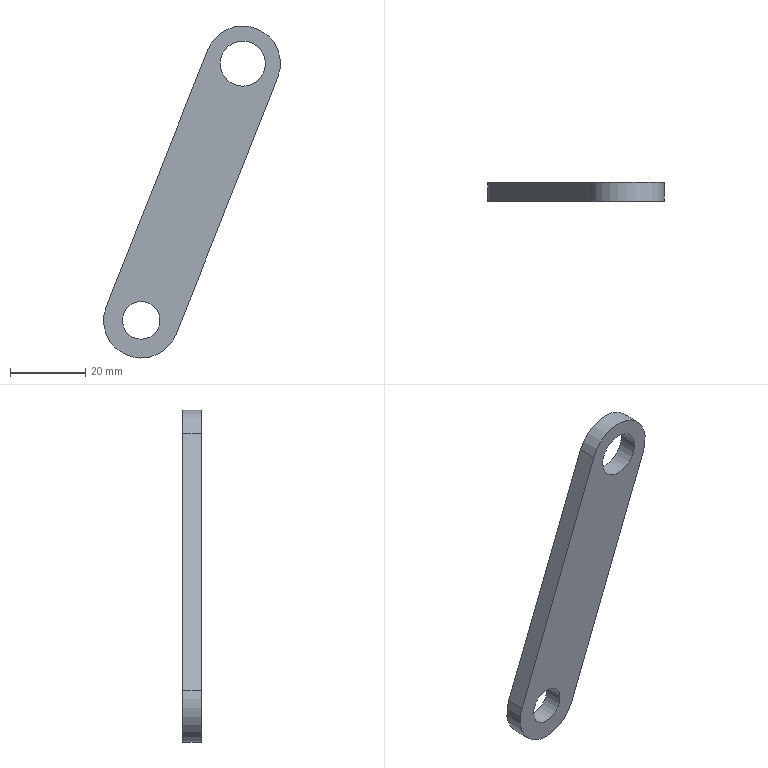Part | STEP file | 冲床-300配套压波_id290_x_t | 1 solid | 8 faces | box 47 x 5 x 88.25 mm | volume 7952 mm3 | cylinder 4 | plane 4 | commonest cylinder face diameters 20 x2 10 x1 12 x1
STEP:
#1=CARTESIAN_POINT('',(1139.299,-32.,157.071));
#2=VERTEX_POINT('',#1);
#3=CARTESIAN_POINT('',(1120.701,-32.,164.429));
#4=VERTEX_POINT('',#3);
#5=CARTESIAN_POINT('',(1130.,-32.,160.75));
#6=DIRECTION('',(0.,1.,0.));
#7=DIRECTION('',(1.,0.,0.));
#8=AXIS2_PLACEMENT_3D('',#5,#6,#7);
#9=CIRCLE('',#8,10.);
#10=EDGE_CURVE('',#2,#4,#9,.T.);
#11=ORIENTED_EDGE('',*,*,#10,.F.);
#12=CARTESIAN_POINT('',(1139.299,-37.,157.071));
#13=VERTEX_POINT('',#12);
#14=CARTESIAN_POINT('',(1139.299,-37.,157.071));
#15=DIRECTION('',(0.,1.,0.));
#16=VECTOR('',#15,1.);
#17=LINE('',#14,#16);
#18=EDGE_CURVE('',#13,#2,#17,.T.);
#19=ORIENTED_EDGE('',*,*,#18,.F.);
#20=CARTESIAN_POINT('',(1120.701,-37.,164.429));
#21=VERTEX_POINT('',#20);
#22=CARTESIAN_POINT('',(1130.,-37.,160.75));
#23=DIRECTION('',(0.,1.,0.));
#24=DIRECTION('',(1.,0.,0.));
#25=AXIS2_PLACEMENT_3D('',#22,#23,#24);
#26=CIRCLE('',#25,10.);
#27=EDGE_CURVE('',#13,#21,#26,.T.);
#28=ORIENTED_EDGE('',*,*,#27,.T.);
#29=CARTESIAN_POINT('',(1120.701,-37.,164.429));
#30=DIRECTION('',(0.,1.,0.));
#31=VECTOR('',#30,1.);
#32=LINE('',#29,#31);
#33=EDGE_CURVE('',#21,#4,#32,.T.);
#34=ORIENTED_EDGE('',*,*,#33,.T.);
#35=EDGE_LOOP('',(#11,#19,#28,#34));
#36=FACE_OUTER_BOUND('',#35,.T.);
#37=CARTESIAN_POINT('',(1130.,-37.,160.75));
#38=DIRECTION('',(0.,1.,0.));
#39=DIRECTION('',(0.,0.,1.));
#40=AXIS2_PLACEMENT_3D('',#37,#38,#39);
#41=CYLINDRICAL_SURFACE('',#40,10.);
#42=ADVANCED_FACE('',(#36),#41,.T.);
#43=CARTESIAN_POINT('',(1147.701,-32.,232.679));
#44=VERTEX_POINT('',#43);
#45=CARTESIAN_POINT('',(1120.701,-32.,164.429));
#46=DIRECTION('',(0.3679,0.,0.9299));
#47=VECTOR('',#46,1.);
#48=LINE('',#45,#47);
#49=EDGE_CURVE('',#4,#44,#48,.T.);
#50=ORIENTED_EDGE('',*,*,#49,.F.);
#51=ORIENTED_EDGE('',*,*,#33,.F.);
#52=CARTESIAN_POINT('',(1147.701,-37.,232.679));
#53=VERTEX_POINT('',#52);
#54=CARTESIAN_POINT('',(1120.701,-37.,164.429));
#55=DIRECTION('',(0.3679,0.,0.9299));
#56=VECTOR('',#55,1.);
#57=LINE('',#54,#56);
#58=EDGE_CURVE('',#21,#53,#57,.T.);
#59=ORIENTED_EDGE('',*,*,#58,.T.);
#60=CARTESIAN_POINT('',(1147.701,-37.,232.679));
#61=DIRECTION('',(0.,1.,0.));
#62=VECTOR('',#61,1.);
#63=LINE('',#60,#62);
#64=EDGE_CURVE('',#53,#44,#63,.T.);
#65=ORIENTED_EDGE('',*,*,#64,.T.);
#66=EDGE_LOOP('',(#50,#51,#59,#65));
#67=FACE_OUTER_BOUND('',#66,.T.);
#68=CARTESIAN_POINT('',(1120.701,-37.,164.429));
#69=DIRECTION('',(-0.9299,0.,0.3679));
#70=DIRECTION('',(0.3679,0.,0.9299));
#71=AXIS2_PLACEMENT_3D('',#68,#69,#70);
#72=PLANE('',#71);
#73=ADVANCED_FACE('',(#67),#72,.T.);
#74=CARTESIAN_POINT('',(1166.299,-32.,225.321));
#75=VERTEX_POINT('',#74);
#76=CARTESIAN_POINT('',(1157.,-32.,229.));
#77=DIRECTION('',(0.,1.,0.));
#78=DIRECTION('',(1.,0.,0.));
#79=AXIS2_PLACEMENT_3D('',#76,#77,#78);
#80=CIRCLE('',#79,10.);
#81=EDGE_CURVE('',#44,#75,#80,.T.);
#82=ORIENTED_EDGE('',*,*,#81,.F.);
#83=ORIENTED_EDGE('',*,*,#64,.F.);
#84=CARTESIAN_POINT('',(1166.299,-37.,225.321));
#85=VERTEX_POINT('',#84);
#86=CARTESIAN_POINT('',(1157.,-37.,229.));
#87=DIRECTION('',(0.,1.,0.));
#88=DIRECTION('',(1.,0.,0.));
#89=AXIS2_PLACEMENT_3D('',#86,#87,#88);
#90=CIRCLE('',#89,10.);
#91=EDGE_CURVE('',#53,#85,#90,.T.);
#92=ORIENTED_EDGE('',*,*,#91,.T.);
#93=CARTESIAN_POINT('',(1166.299,-37.,225.321));
#94=DIRECTION('',(0.,1.,0.));
#95=VECTOR('',#94,1.);
#96=LINE('',#93,#95);
#97=EDGE_CURVE('',#85,#75,#96,.T.);
#98=ORIENTED_EDGE('',*,*,#97,.T.);
#99=EDGE_LOOP('',(#82,#83,#92,#98));
#100=FACE_OUTER_BOUND('',#99,.T.);
#101=CARTESIAN_POINT('',(1157.,-37.,229.));
#102=DIRECTION('',(0.,1.,0.));
#103=DIRECTION('',(0.,0.,1.));
#104=AXIS2_PLACEMENT_3D('',#101,#102,#103);
#105=CYLINDRICAL_SURFACE('',#104,10.);
#106=ADVANCED_FACE('',(#100),#105,.T.);
#107=CARTESIAN_POINT('',(1166.299,-32.,225.321));
#108=DIRECTION('',(-0.3679,0.,-0.9299));
#109=VECTOR('',#108,1.);
#110=LINE('',#107,#109);
#111=EDGE_CURVE('',#75,#2,#110,.T.);
#112=ORIENTED_EDGE('',*,*,#111,.F.);
#113=ORIENTED_EDGE('',*,*,#97,.F.);
#114=CARTESIAN_POINT('',(1166.299,-37.,225.321));
#115=DIRECTION('',(-0.3679,0.,-0.9299));
#116=VECTOR('',#115,1.);
#117=LINE('',#114,#116);
#118=EDGE_CURVE('',#85,#13,#117,.T.);
#119=ORIENTED_EDGE('',*,*,#118,.T.);
#120=ORIENTED_EDGE('',*,*,#18,.T.);
#121=EDGE_LOOP('',(#112,#113,#119,#120));
#122=FACE_OUTER_BOUND('',#121,.T.);
#123=CARTESIAN_POINT('',(1166.299,-37.,225.321));
#124=DIRECTION('',(0.9299,0.,-0.3679));
#125=DIRECTION('',(-0.3679,0.,-0.9299));
#126=AXIS2_PLACEMENT_3D('',#123,#124,#125);
#127=PLANE('',#126);
#128=ADVANCED_FACE('',(#122),#127,.T.);
#129=CARTESIAN_POINT('',(1130.,-37.,165.75));
#130=VERTEX_POINT('',#129);
#131=CARTESIAN_POINT('',(1130.,-37.,160.75));
#132=DIRECTION('',(0.,-1.,0.));
#133=DIRECTION('',(0.,0.,1.));
#134=AXIS2_PLACEMENT_3D('',#131,#132,#133);
#135=CIRCLE('',#134,5.);
#136=EDGE_CURVE('',#130,#130,#135,.T.);
#137=ORIENTED_EDGE('',*,*,#136,.F.);
#138=EDGE_LOOP('',(#137));
#139=FACE_BOUND('',#138,.T.);
#140=CARTESIAN_POINT('',(1157.,-37.,235.));
#141=VERTEX_POINT('',#140);
#142=CARTESIAN_POINT('',(1157.,-37.,229.));
#143=DIRECTION('',(0.,-1.,0.));
#144=DIRECTION('',(0.,0.,1.));
#145=AXIS2_PLACEMENT_3D('',#142,#143,#144);
#146=CIRCLE('',#145,6.);
#147=EDGE_CURVE('',#141,#141,#146,.T.);
#148=ORIENTED_EDGE('',*,*,#147,.F.);
#149=EDGE_LOOP('',(#148));
#150=FACE_BOUND('',#149,.T.);
#151=ORIENTED_EDGE('',*,*,#27,.F.);
#152=ORIENTED_EDGE('',*,*,#118,.F.);
#153=ORIENTED_EDGE('',*,*,#91,.F.);
#154=ORIENTED_EDGE('',*,*,#58,.F.);
#155=EDGE_LOOP('',(#151,#152,#153,#154));
#156=FACE_BOUND('',#155,.T.);
#157=CARTESIAN_POINT('',(1130.,-37.,160.75));
#158=DIRECTION('',(0.,1.,0.));
#159=DIRECTION('',(0.,0.,1.));
#160=AXIS2_PLACEMENT_3D('',#157,#158,#159);
#161=PLANE('',#160);
#162=ADVANCED_FACE('',(#139,#150,#156),#161,.F.);
#163=ORIENTED_EDGE('',*,*,#111,.T.);
#164=ORIENTED_EDGE('',*,*,#10,.T.);
#165=ORIENTED_EDGE('',*,*,#49,.T.);
#166=ORIENTED_EDGE('',*,*,#81,.T.);
#167=EDGE_LOOP('',(#163,#164,#165,#166));
#168=FACE_BOUND('',#167,.T.);
#169=CARTESIAN_POINT('',(1157.,-32.,235.));
#170=VERTEX_POINT('',#169);
#171=CARTESIAN_POINT('',(1157.,-32.,229.));
#172=DIRECTION('',(0.,-1.,0.));
#173=DIRECTION('',(0.,0.,1.));
#174=AXIS2_PLACEMENT_3D('',#171,#172,#173);
#175=CIRCLE('',#174,6.);
#176=EDGE_CURVE('',#170,#170,#175,.T.);
#177=ORIENTED_EDGE('',*,*,#176,.T.);
#178=EDGE_LOOP('',(#177));
#179=FACE_BOUND('',#178,.T.);
#180=CARTESIAN_POINT('',(1130.,-32.,155.75));
#181=VERTEX_POINT('',#180);
#182=CARTESIAN_POINT('',(1130.,-32.,160.75));
#183=DIRECTION('',(0.,-1.,0.));
#184=DIRECTION('',(0.,0.,-1.));
#185=AXIS2_PLACEMENT_3D('',#182,#183,#184);
#186=CIRCLE('',#185,5.);
#187=EDGE_CURVE('',#181,#181,#186,.T.);
#188=ORIENTED_EDGE('',*,*,#187,.T.);
#189=EDGE_LOOP('',(#188));
#190=FACE_BOUND('',#189,.T.);
#191=CARTESIAN_POINT('',(1130.,-32.,160.75));
#192=DIRECTION('',(0.,1.,0.));
#193=DIRECTION('',(0.,0.,1.));
#194=AXIS2_PLACEMENT_3D('',#191,#192,#193);
#195=PLANE('',#194);
#196=ADVANCED_FACE('',(#168,#179,#190),#195,.T.);
#197=ORIENTED_EDGE('',*,*,#176,.F.);
#198=EDGE_LOOP('',(#197));
#199=FACE_BOUND('',#198,.T.);
#200=ORIENTED_EDGE('',*,*,#147,.T.);
#201=EDGE_LOOP('',(#200));
#202=FACE_BOUND('',#201,.T.);
#203=CARTESIAN_POINT('',(1157.,60.,229.));
#204=DIRECTION('',(0.,-1.,0.));
#205=DIRECTION('',(0.,0.,-1.));
#206=AXIS2_PLACEMENT_3D('',#203,#204,#205);
#207=CYLINDRICAL_SURFACE('',#206,6.);
#208=ADVANCED_FACE('',(#199,#202),#207,.F.);
#209=ORIENTED_EDGE('',*,*,#187,.F.);
#210=EDGE_LOOP('',(#209));
#211=FACE_BOUND('',#210,.T.);
#212=ORIENTED_EDGE('',*,*,#136,.T.);
#213=EDGE_LOOP('',(#212));
#214=FACE_BOUND('',#213,.T.);
#215=CARTESIAN_POINT('',(1130.,-65.,160.75));
#216=DIRECTION('',(0.,1.,0.));
#217=DIRECTION('',(0.,0.,1.));
#218=AXIS2_PLACEMENT_3D('',#215,#216,#217);
#219=CYLINDRICAL_SURFACE('',#218,5.);
#220=ADVANCED_FACE('',(#211,#214),#219,.F.);
#221=CLOSED_SHELL('',(#42,#73,#106,#128,#162,#196,#208,#220));
#222=MANIFOLD_SOLID_BREP('',#221);
#223=(LENGTH_UNIT()NAMED_UNIT(*)SI_UNIT(.MILLI.,.METRE.));
#224=UNCERTAINTY_MEASURE_WITH_UNIT(LENGTH_MEASURE(0.00002),#223,'','');
#225=(NAMED_UNIT(*)PLANE_ANGLE_UNIT()SI_UNIT($,.RADIAN.));
#226=PLANE_ANGLE_MEASURE_WITH_UNIT(PLANE_ANGLE_MEASURE(0.01745),#225);
#227=DIMENSIONAL_EXPONENTS(0.,0.,0.,0.,0.,0.,0.);
#228=(CONVERSION_BASED_UNIT('DEGREE',#226)NAMED_UNIT(#227)PLANE_ANGLE_UNIT());
#229=(NAMED_UNIT(*)SI_UNIT($,.STERADIAN.)SOLID_ANGLE_UNIT());
#230=(GEOMETRIC_REPRESENTATION_CONTEXT(3)GLOBAL_UNCERTAINTY_ASSIGNED_CONTEXT((#224))GLOBAL_UNIT_ASSIGNED_CONTEXT((#223,#228,#229))REPRESENTATION_CONTEXT('',''));
#231=ADVANCED_BREP_SHAPE_REPRESENTATION('',(#222),#230);